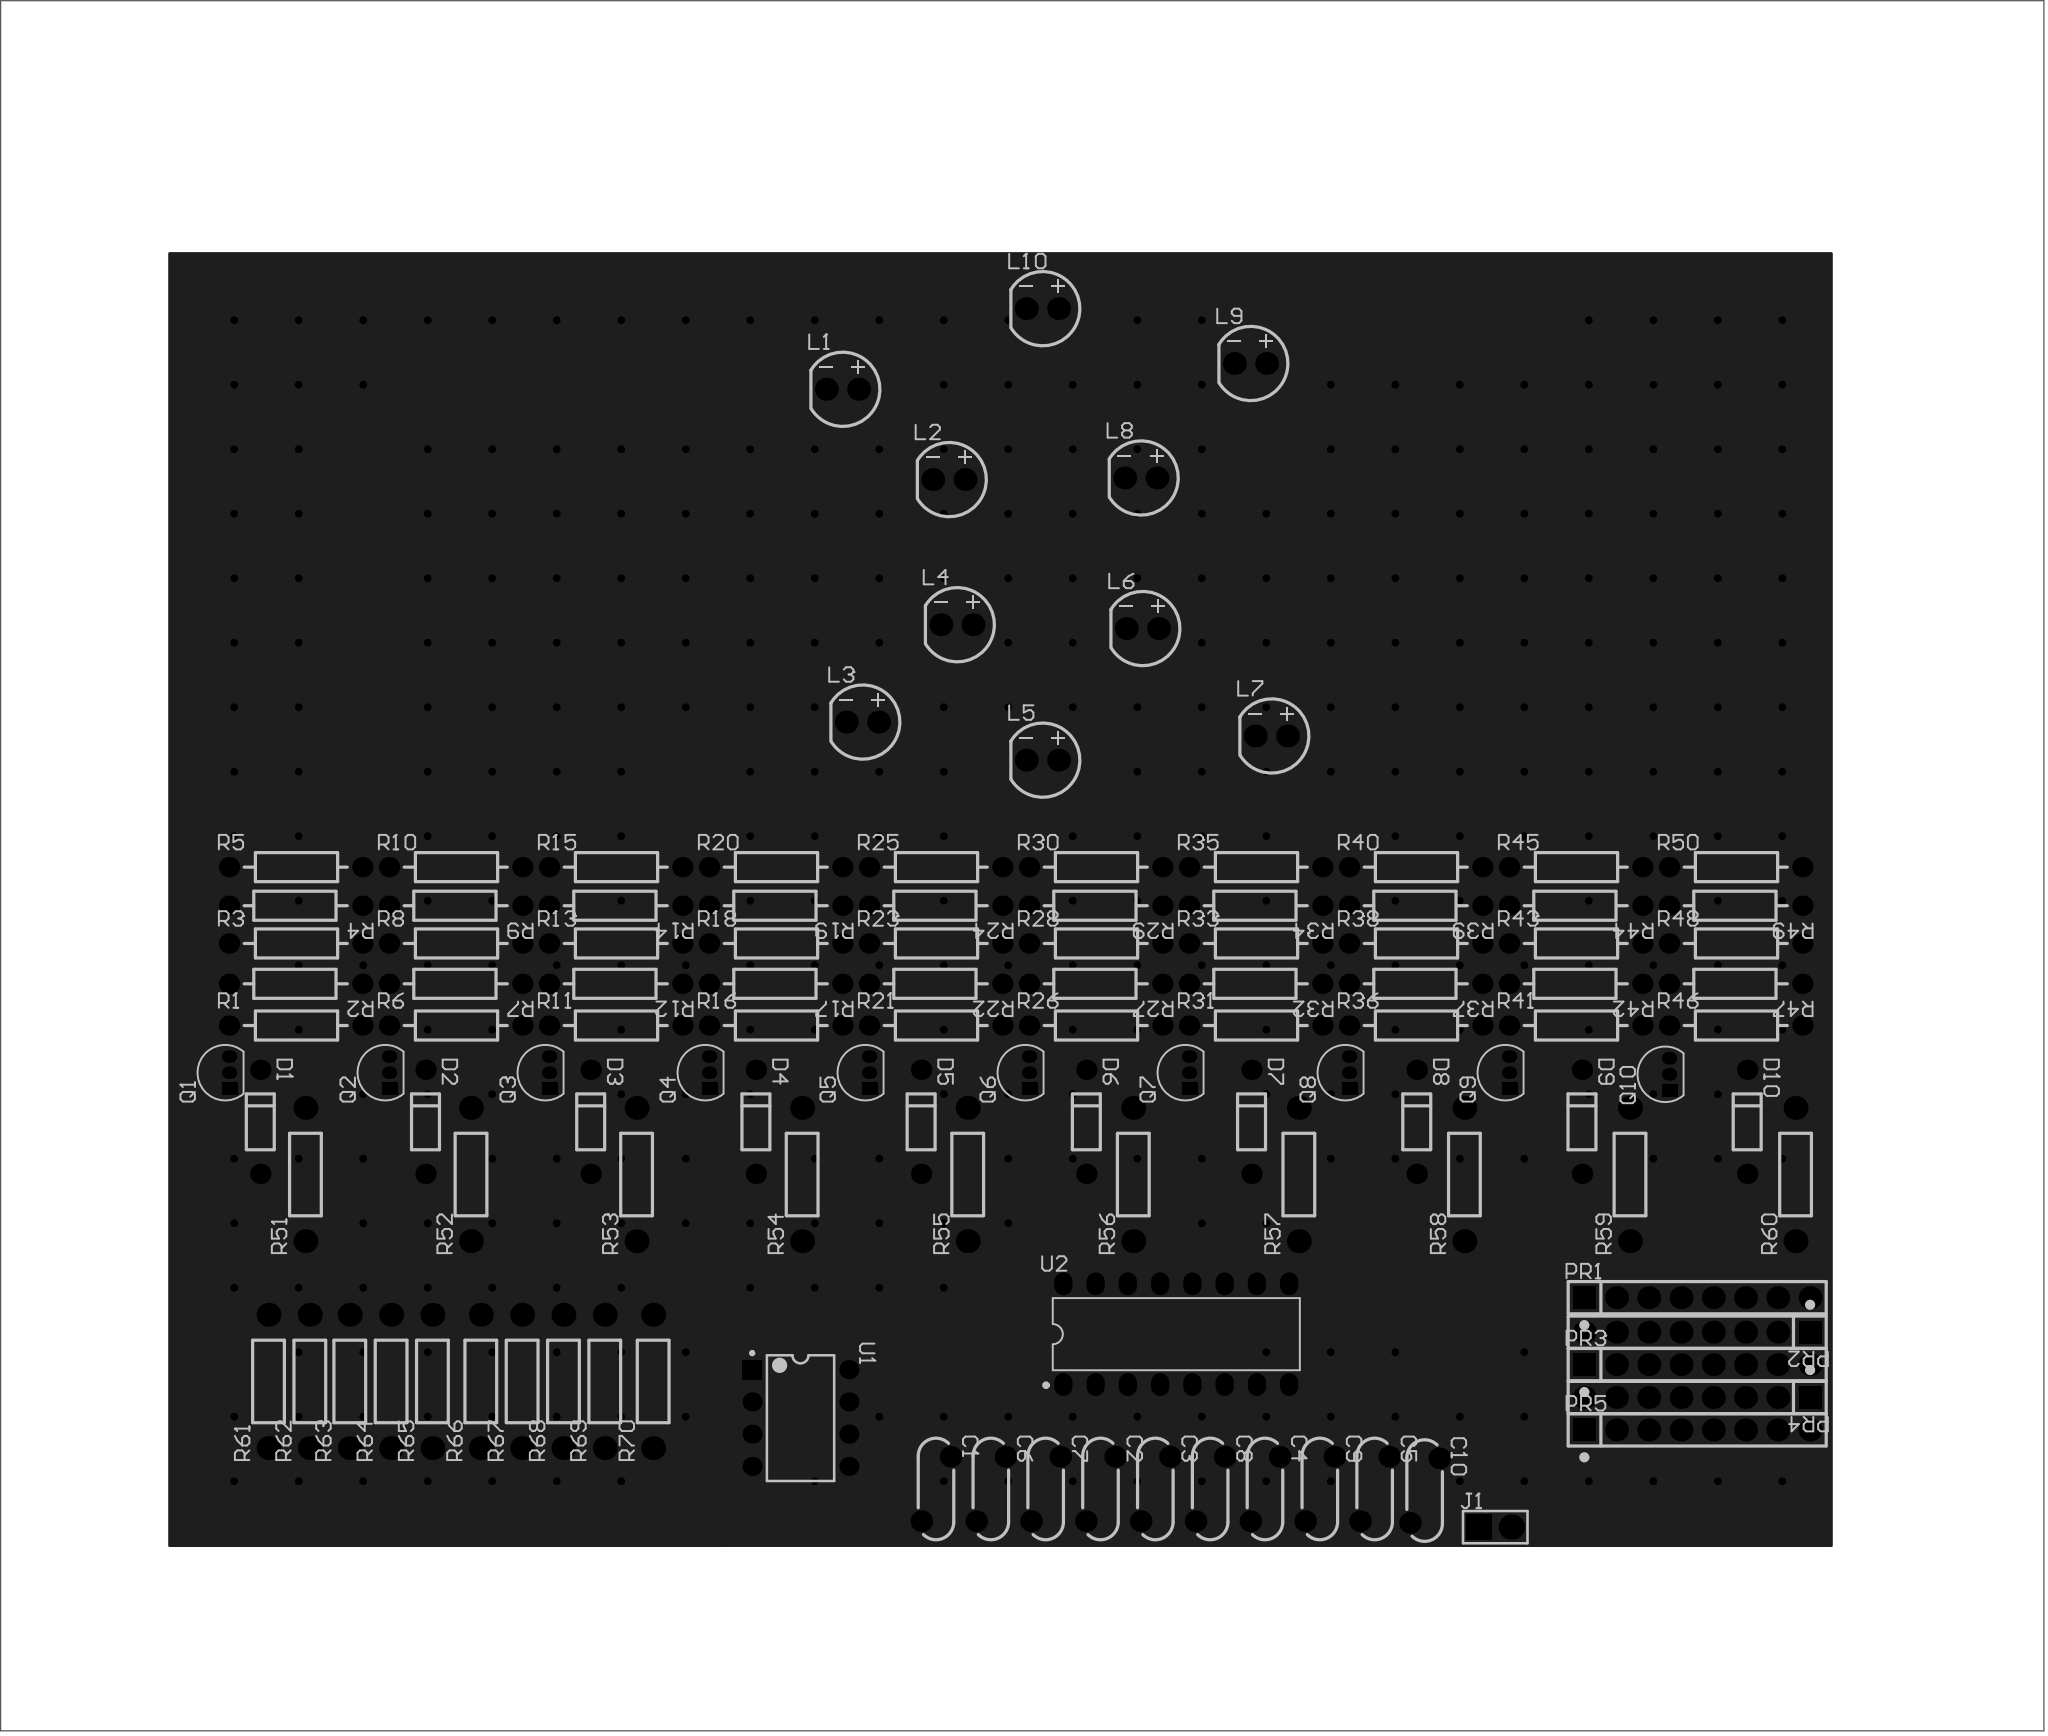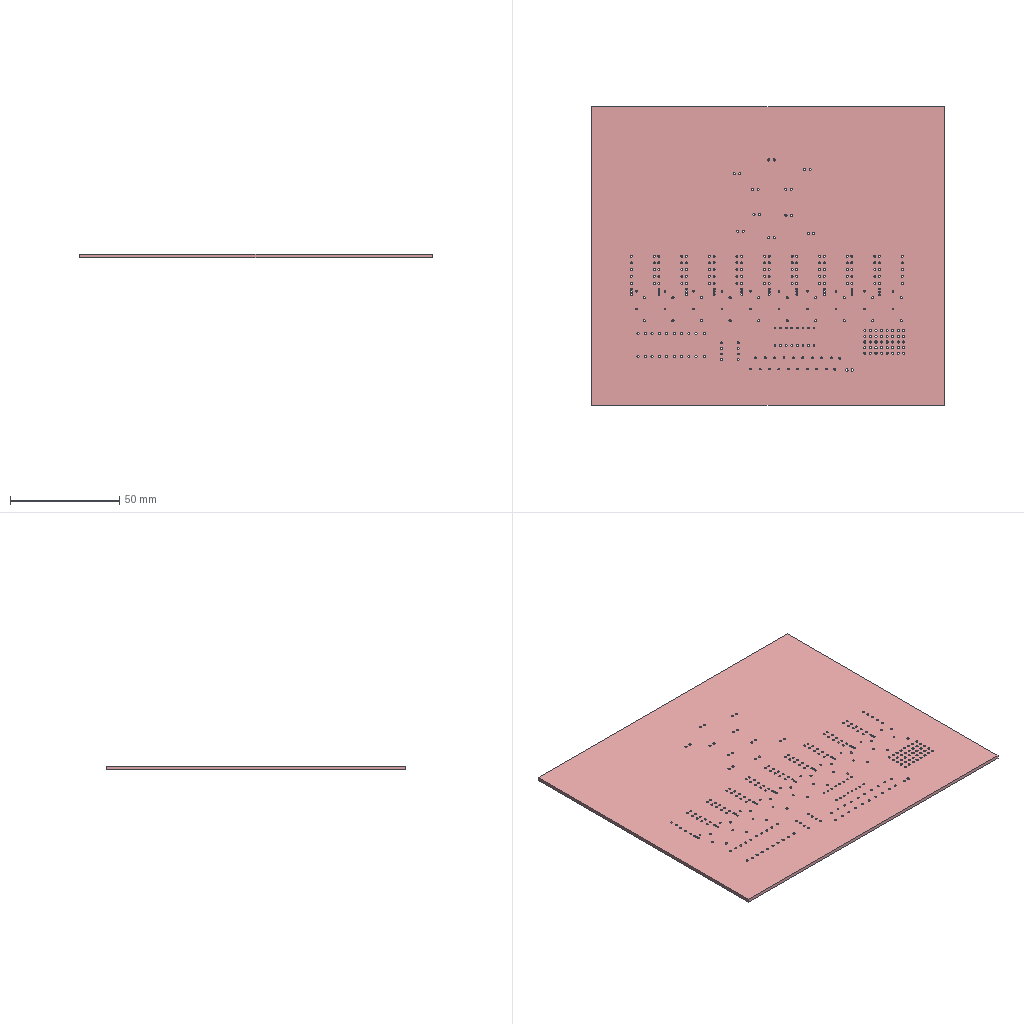Circuit board layout | Altium Designer | box 160.9 x 136.3 x 1.6 mm
Layer stack:
# Altium Designer layer stack of  (unit mm; dielectric type: 0 none, 1 core, 2 prepreg, 3 surface material)
index,name,kind,layer,copper_thickness_mm,dielectric_type,dielectric_thickness_mm,dielectric_material,dielectric_constant
0,Top Paste Mask Layer,other,,,,,,
1,Top Silkscreen Layer,other,,,,,,
2,Top Solder Mask Layer,dielectric,,,3,0.01,,3.3
3,Top Layer,copper,Top Layer,0.035,,,,
4,Dielectric1,dielectric,,,3,1.51,FR4,4.5
5,Bottom Layer,copper,Bottom Layer,0.035,,,,
6,Bottom Solder Mask Layer,dielectric,,,3,0.01,,3.3
7,Bottom Silkscreen Layer,other,,,,,,
8,Bottom Paste Mask Layer,other,,,,,,
# drill layer pairs: low layer,high layer
drill_pair,Top Layer,Bottom Layer
Part placement:
Designator,Comment,Layer,Footprint,Center-X(mm),Center-Y(mm),Rotation
C1,10nF,TopLayer,CAP-TH_L8.0-W2.8-P5.08-D0.6,143.51,88.9,270
C2,10nF,TopLayer,CAP-TH_L8.0-W2.8-P5.08-D0.6,156.464,88.9,270
C3,10nF,TopLayer,CAP-TH_L8.0-W2.8-P5.08-D0.6,160.782,88.9,270
C4,10nF,TopLayer,CAP-TH_L8.0-W2.8-P5.08-D0.6,169.418,88.9,270
C5,10nF,TopLayer,CAP-TH_L8.0-W2.8-P5.08-D0.6,178.054,88.9,270
C6,10nF,TopLayer,CAP-TH_L8.0-W2.8-P5.08-D0.6,147.828,88.9,270
C7,10nF,TopLayer,CAP-TH_L8.0-W2.8-P5.08-D0.6,152.146,88.9,270
C8,10nF,TopLayer,CAP-TH_L8.0-W2.8-P5.08-D0.6,165.1,88.9,270
C9,10nF,TopLayer,CAP-TH_L8.0-W2.8-P5.08-D0.6,173.736,88.9,270
C10,10nF,TopLayer,CAP-TH_L8.0-W2.8-P5.08-D0.6,181.991,88.773,270
D1,1N4148TR,TopLayer,DO-35_BD2.0-L4.2-P8.20-D0.5-RD,90.297,117.815,270
D2,1N4148TR,TopLayer,DO-35_BD2.0-L4.2-P8.20-D0.5-RD,103.307,117.815,270
D3,1N4148TR,TopLayer,DO-35_BD2.0-L4.2-P8.20-D0.5-RD,116.318,117.815,270
D4,1N4148TR,TopLayer,DO-35_BD2.0-L4.2-P8.20-D0.5-RD,129.328,117.815,270
D5,1N4148TR,TopLayer,DO-35_BD2.0-L4.2-P8.20-D0.5-RD,142.339,117.815,270
D6,1N4148TR,TopLayer,DO-35_BD2.0-L4.2-P8.20-D0.5-RD,155.349,117.815,270
D7,1N4148TR,TopLayer,DO-35_BD2.0-L4.2-P8.20-D0.5-RD,168.36,117.815,270
D8,1N4148TR,TopLayer,DO-35_BD2.0-L4.2-P8.20-D0.5-RD,181.37,117.815,270
D9,1N4148TR,TopLayer,DO-35_BD2.0-L4.2-P8.20-D0.5-RD,194.381,117.815,270
D10,1N4148TR,TopLayer,DO-35_BD2.0-L4.2-P8.20-D0.5-RD,207.391,117.815,270
J1,PZ254V-11-02P,TopLayer,HDR-TH_2P-P2.54-V-M,187.552,85.892,0
L1,XL-502SURD,TopLayer,LED-TH_BD5.9-P2.54-RD_RED,136.144,175.514,0
L2,XL-502SURD,TopLayer,LED-TH_BD5.9-P2.54-RD_RED,144.526,168.402,0
L3,XL-502SURD,TopLayer,LED-TH_BD5.9-P2.54-RD_RED,137.718,149.303,0
L4,XL-502SURD,TopLayer,LED-TH_BD5.9-P2.54-RD_RED,145.161,156.972,0
L5,XL-502SURD,TopLayer,LED-TH_BD5.9-P2.54-RD_RED,151.892,146.304,0
L6,XL-502SURD,TopLayer,LED-TH_BD5.9-P2.54-RD_RED,159.771,156.669,0
L7,XL-502SURD,TopLayer,LED-TH_BD5.9-P2.54-RD_RED,169.926,148.209,0
L8,XL-502SURD,TopLayer,LED-TH_BD5.9-P2.54-RD_RED,159.639,168.529,0
L9,XL-502SURD,TopLayer,LED-TH_BD5.9-P2.54-RD_RED,168.275,177.546,0
L10,XL-502SURD,TopLayer,LED-TH_BD5.9-P2.54-RD_RED,151.892,181.864,0
PR1,10kΩ,TopLayer,RES-ARRAY-TH_8P-L20.3-W2.5-P2.54,203.454,103.964,0
PR2,10kΩ,TopLayer,RES-ARRAY-TH_8P-L20.3-W2.5-P2.54,203.454,101.247,180
PR3,10kΩ,TopLayer,RES-ARRAY-TH_8P-L20.3-W2.5-P2.54,203.454,98.695,0
PR4,10kΩ,TopLayer,RES-ARRAY-TH_8P-L20.3-W2.5-P2.54,203.454,96.105,180
PR5,10kΩ,TopLayer,RES-ARRAY-TH_8P-L20.3-W2.5-P2.54,203.454,93.552,0
Q1,S8050,TopLayer,TO-92-3_L4.5-W3.5-P1.27-L,87.88,121.686,90
Q2,S8050,TopLayer,TO-92-3_L4.5-W3.5-P1.27-L,100.48,121.686,90
Q3,S8050,TopLayer,TO-92-3_L4.5-W3.5-P1.27-L,113.08,121.686,90
Q4,S8050,TopLayer,TO-92-3_L4.5-W3.5-P1.27-L,125.68,121.686,90
Q5,S8050,TopLayer,TO-92-3_L4.5-W3.5-P1.27-L,138.28,121.686,90
Q6,S8050,TopLayer,TO-92-3_L4.5-W3.5-P1.27-L,150.881,121.686,90
Q7,S8050,TopLayer,TO-92-3_L4.5-W3.5-P1.27-L,163.481,121.686,90
Q8,S8050,TopLayer,TO-92-3_L4.5-W3.5-P1.27-L,176.081,121.686,90
Q9,S8050,TopLayer,TO-92-3_L4.5-W3.5-P1.27-L,188.681,121.686,90
Q10,S8050,TopLayer,TO-92-3_L4.5-W3.5-P1.27-L,201.281,121.559,90
R1,100Ω,TopLayer,RES-TH_BD2.2-L6.5-P10.50-D0.6,93.087,125.402,0
R2,100Ω,TopLayer,RES-TH_BD2.2-L6.5-P10.50-D0.6,93.087,128.687,180
R3,100Ω,TopLayer,RES-TH_BD2.2-L6.5-P10.50-D0.6,93.087,131.865,0
R4,100Ω,TopLayer,RES-TH_BD2.2-L6.5-P10.50-D0.6,93.087,134.837,180
R5,100Ω,TopLayer,RES-TH_BD2.2-L6.5-P10.50-D0.6,93.087,137.877,0
R6,100Ω,TopLayer,RES-TH_BD2.2-L6.5-P10.50-D0.6,105.687,125.402,0
R7,100Ω,TopLayer,RES-TH_BD2.2-L6.5-P10.50-D0.6,105.687,128.687,180
R8,100Ω,TopLayer,RES-TH_BD2.2-L6.5-P10.50-D0.6,105.687,131.865,0
R9,100Ω,TopLayer,RES-TH_BD2.2-L6.5-P10.50-D0.6,105.687,134.837,180
R10,100Ω,TopLayer,RES-TH_BD2.2-L6.5-P10.50-D0.6,105.687,137.877,0
R11,100Ω,TopLayer,RES-TH_BD2.2-L6.5-P10.50-D0.6,118.287,125.402,0
R12,100Ω,TopLayer,RES-TH_BD2.2-L6.5-P10.50-D0.6,118.287,128.687,180
R13,100Ω,TopLayer,RES-TH_BD2.2-L6.5-P10.50-D0.6,118.287,131.865,0
R14,100Ω,TopLayer,RES-TH_BD2.2-L6.5-P10.50-D0.6,118.287,134.837,180
R15,100Ω,TopLayer,RES-TH_BD2.2-L6.5-P10.50-D0.6,118.287,137.877,0
R16,100Ω,TopLayer,RES-TH_BD2.2-L6.5-P10.50-D0.6,130.887,125.402,0
R17,100Ω,TopLayer,RES-TH_BD2.2-L6.5-P10.50-D0.6,130.887,128.687,180
R18,100Ω,TopLayer,RES-TH_BD2.2-L6.5-P10.50-D0.6,130.887,131.865,0
R19,100Ω,TopLayer,RES-TH_BD2.2-L6.5-P10.50-D0.6,130.887,134.837,180
R20,100Ω,TopLayer,RES-TH_BD2.2-L6.5-P10.50-D0.6,130.887,137.877,0
R21,100Ω,TopLayer,RES-TH_BD2.2-L6.5-P10.50-D0.6,143.487,125.402,0
R22,100Ω,TopLayer,RES-TH_BD2.2-L6.5-P10.50-D0.6,143.488,128.687,180
R23,100Ω,TopLayer,RES-TH_BD2.2-L6.5-P10.50-D0.6,143.487,131.865,0
R24,100Ω,TopLayer,RES-TH_BD2.2-L6.5-P10.50-D0.6,143.488,134.837,180
R25,100Ω,TopLayer,RES-TH_BD2.2-L6.5-P10.50-D0.6,143.487,137.877,0
R26,100Ω,TopLayer,RES-TH_BD2.2-L6.5-P10.50-D0.6,156.088,125.402,0
R27,100Ω,TopLayer,RES-TH_BD2.2-L6.5-P10.50-D0.6,156.088,128.687,180
R28,100Ω,TopLayer,RES-TH_BD2.2-L6.5-P10.50-D0.6,156.088,131.865,0
R29,100Ω,TopLayer,RES-TH_BD2.2-L6.5-P10.50-D0.6,156.088,134.837,180
R30,100Ω,TopLayer,RES-TH_BD2.2-L6.5-P10.50-D0.6,156.088,137.877,0
R31,100Ω,TopLayer,RES-TH_BD2.2-L6.5-P10.50-D0.6,168.688,125.402,0
R32,100Ω,TopLayer,RES-TH_BD2.2-L6.5-P10.50-D0.6,168.688,128.687,180
R33,100Ω,TopLayer,RES-TH_BD2.2-L6.5-P10.50-D0.6,168.688,131.865,0
R34,100Ω,TopLayer,RES-TH_BD2.2-L6.5-P10.50-D0.6,168.688,134.837,180
R35,100Ω,TopLayer,RES-TH_BD2.2-L6.5-P10.50-D0.6,168.688,137.877,0
R36,100Ω,TopLayer,RES-TH_BD2.2-L6.5-P10.50-D0.6,181.288,125.402,0
R37,100Ω,TopLayer,RES-TH_BD2.2-L6.5-P10.50-D0.6,181.288,128.687,180
R38,100Ω,TopLayer,RES-TH_BD2.2-L6.5-P10.50-D0.6,181.288,131.865,0
R39,100Ω,TopLayer,RES-TH_BD2.2-L6.5-P10.50-D0.6,181.288,134.837,180
R40,100Ω,TopLayer,RES-TH_BD2.2-L6.5-P10.50-D0.6,181.288,137.877,0
R41,100Ω,TopLayer,RES-TH_BD2.2-L6.5-P10.50-D0.6,193.888,125.402,0
R42,100Ω,TopLayer,RES-TH_BD2.2-L6.5-P10.50-D0.6,193.888,128.687,180
R43,100Ω,TopLayer,RES-TH_BD2.2-L6.5-P10.50-D0.6,193.888,131.865,0
R44,100Ω,TopLayer,RES-TH_BD2.2-L6.5-P10.50-D0.6,193.888,134.837,180
R45,100Ω,TopLayer,RES-TH_BD2.2-L6.5-P10.50-D0.6,193.888,137.877,0
R46,100Ω,TopLayer,RES-TH_BD2.2-L6.5-P10.50-D0.6,206.488,125.402,0
R47,100Ω,TopLayer,RES-TH_BD2.2-L6.5-P10.50-D0.6,206.488,128.687,180
R48,100Ω,TopLayer,RES-TH_BD2.2-L6.5-P10.50-D0.6,206.488,131.865,0
R49,100Ω,TopLayer,RES-TH_BD2.2-L6.5-P10.50-D0.6,206.488,134.837,180
R50,100Ω,TopLayer,RES-TH_BD2.2-L6.5-P10.50-D0.6,206.488,137.877,0
R51,1kΩ,TopLayer,RES-TH_BD2.5-L6.5-P10.50-D0.6,93.853,113.665,90
R52,1kΩ,TopLayer,RES-TH_BD2.5-L6.5-P10.50-D0.6,106.892,113.665,90
R53,1kΩ,TopLayer,RES-TH_BD2.5-L6.5-P10.50-D0.6,119.93,113.665,90
R54,1kΩ,TopLayer,RES-TH_BD2.5-L6.5-P10.50-D0.6,132.969,113.665,90
R55,1kΩ,TopLayer,RES-TH_BD2.5-L6.5-P10.50-D0.6,146.008,113.665,90
R56,1kΩ,TopLayer,RES-TH_BD2.5-L6.5-P10.50-D0.6,159.046,113.665,90
R57,1kΩ,TopLayer,RES-TH_BD2.5-L6.5-P10.50-D0.6,172.085,113.665,90
R58,1kΩ,TopLayer,RES-TH_BD2.5-L6.5-P10.50-D0.6,185.124,113.665,90
R59,1kΩ,TopLayer,RES-TH_BD2.5-L6.5-P10.50-D0.6,198.162,113.665,90
R60,1kΩ,TopLayer,RES-TH_BD2.5-L6.5-P10.50-D0.6,211.201,113.665,90
R61,1kΩ,TopLayer,RES-TH_BD2.5-L6.5-P10.50-D0.6,90.944,97.368,90
R62,1kΩ,TopLayer,RES-TH_BD2.5-L6.5-P10.50-D0.6,94.198,97.368,90
R63,1kΩ,TopLayer,RES-TH_BD2.5-L6.5-P10.50-D0.6,97.346,97.368,90
R64,1kΩ,TopLayer,RES-TH_BD2.5-L6.5-P10.50-D0.6,100.6,97.368,90
R65,1kΩ,TopLayer,RES-TH_BD2.5-L6.5-P10.50-D0.6,103.853,97.368,90
R66,1kΩ,TopLayer,RES-TH_BD2.5-L6.5-P10.50-D0.6,107.663,97.368,90
R67,1kΩ,TopLayer,RES-TH_BD2.5-L6.5-P10.50-D0.6,110.918,97.368,90
R68,1kΩ,TopLayer,RES-TH_BD2.5-L6.5-P10.50-D0.6,114.172,97.368,90
R69,1kΩ,TopLayer,RES-TH_BD2.5-L6.5-P10.50-D0.6,117.426,97.368,90
R70,1kΩ,TopLayer,RES-TH_BD2.5-L6.5-P10.50-D0.6,121.236,97.368,90
U1,NE555P,TopLayer,DIP-8_L9.8-W6.6-P2.54-LS7.6-BL,132.842,94.488,270
U2,CD4017CN,TopLayer,PDIP-16_L19.3-W6.4-P2.54-LS7.94-BL,162.433,101.092,0
Pad and via stacks:
# Altium Designer via and pad stacks of  (unit mm). Each distinct definition once, with the count of objects using it.
# via: kind,start_layer,end_layer,hole_mm,diameter_mm,mode(0 simple;1 top-mid-bottom;2 full stack),diameter_per_layer,count,example_net
# pad: kind,layer,hole_mm,hole_type(0 round;1 square;2 slot),plating,top_size,top_shape(1 round;2 rect;3 octagon;9 rounded rect),mid_size,bottom_size,mode,footprint,size_per_layer,count,example
pad,Multi-Layer,0.9,0,plated,1.7x1.7,1,1.7x1.7,1.7x1.7,0,CAP-TH_L8.0-W2.8-P5.08-D0.6,,20,C1.1
pad,Multi-Layer,0.8,0,plated,1.6x1.6,1,1.6x1.6,1.6x1.6,0,DO-35_BD2.0-L4.2-P8.20-D0.5-RD,,20,D1.2
pad,Multi-Layer,1.2,0,plated,2x2,2,2x2,2x2,0,HDR-TH_2P-P2.54-V-M,,1,J1.1
pad,Multi-Layer,1.2,0,plated,2x2,1,2x2,2x2,0,HDR-TH_2P-P2.54-V-M,,1,J1.2
pad,Multi-Layer,1,0,plated,1.8x1.8,1,1.8x1.8,1.8x1.8,0,LED-TH_BD5.9-P2.54-RD_RED,,20,L1.2
pad,Multi-Layer,1,0,plated,1.8x1.8,2,1.8x1.8,1.8x1.8,0,RES-ARRAY-TH_8P-L20.3-W2.5-P2.54,,5,PR1.1
pad,Multi-Layer,1,0,plated,1.8x1.8,1,1.8x1.8,1.8x1.8,0,RES-ARRAY-TH_8P-L20.3-W2.5-P2.54,,35,PR1.2
pad,Multi-Layer,0.7,2,plated,1x1.2,2,1x1.2,1x1.2,0,TO-92-3_L4.5-W3.5-P1.27-L,,10,Q1.1
pad,Multi-Layer,0.7,2,plated,1x1.2,1,1x1.2,1x1.2,0,TO-92-3_L4.5-W3.5-P1.27-L,,20,Q1.2
pad,Multi-Layer,0.9144,0,plated,1.6x1.6,1,1.6x1.6,1.6x1.6,0,RES-TH_BD2.2-L6.5-P10.50-D0.6,,100,R1.1
pad,Multi-Layer,1,0,plated,1.88x1.88,1,1.88x1.88,1.88x1.88,0,RES-TH_BD2.5-L6.5-P10.50-D0.6,,40,R51.1
pad,Multi-Layer,0.9,0,plated,1.5x1.5,2,1.5x1.5,1.5x1.5,0,DIP-8_L9.8-W6.6-P2.54-LS7.6-BL,,1,U1.1
pad,Multi-Layer,0.9,0,plated,1.5x1.5,1,1.5x1.5,1.5x1.5,0,DIP-8_L9.8-W6.6-P2.54-LS7.6-BL,,7,U1.2
pad,Multi-Layer,0.8,0,plated,1.44x1.8,1,1.44x1.8,1.44x1.8,0,PDIP-16_L19.3-W6.4-P2.54-LS7.94-BL,,16,U2.1
via,Top Layer,Bottom Layer,0.3048,0.61,0,,358,GND
Copper pours:
name,layer,net,type(0 solid;1 hatched;2 none)
Bottom Layer-GND,Bottom Layer,GND,0
Top Layer-GND,Top Layer,GND,0